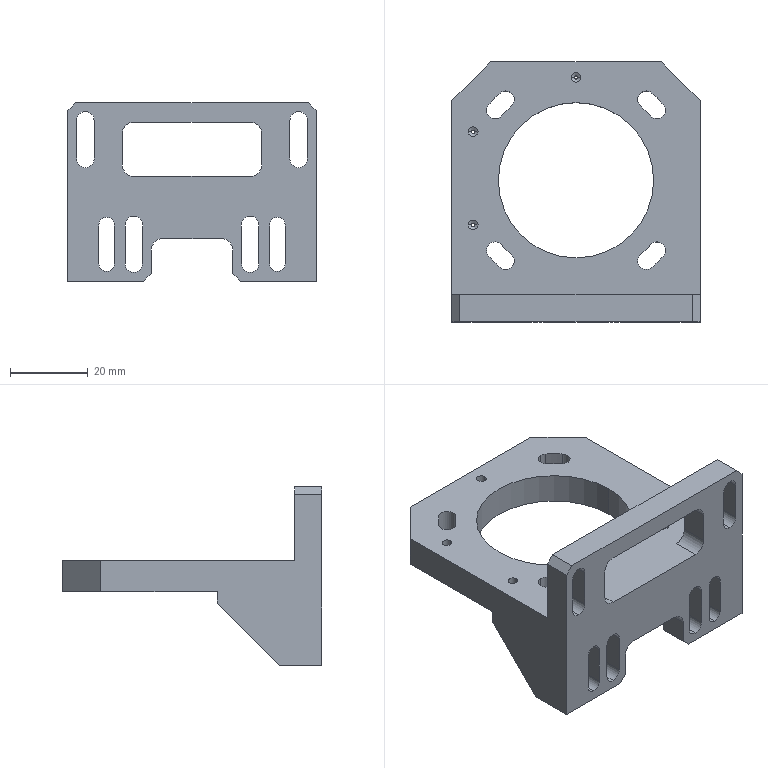NC program | NX | posted with a generic post | part box 64 x 67 x 46 mm
Lines 1 to 517 of 30645:
N10 G17 G21 G94 G90
(FLOOR_WALL_COPY , TOOL : D63)
N12 T02 M6
N14 G54
N16 G17 G0 G90 X-70. Y31.997 B0. C0. S2000 M3
N18 G43 Z30. H2
N20 Z6.9
N22 G94 G1 Z3.9 F1250.
N24 X-65.
N26 X65.
N28 Y12.599
N30 X-65.
N32 Y-6.8
N34 X65.
N36 X70.
N38 Z6.9
N40 G0 Z30.
N42 X-70. Y31.997
N44 Z6.8
N46 G1 Z3.8
N48 X-65.
N50 X65.
N52 Y12.599
N54 X-65.
N56 Y-6.8
N58 X65.
N60 X70.
N62 Z6.8
N64 G0 Z30.
N66 X-70. Y31.997
N68 Z6.7
N70 G1 Z3.7
N72 X-65.
N74 X65.
N76 Y12.599
N78 X-65.
N80 Y-6.8
N82 X65.
N84 X70.
N86 Z6.7
N88 G0 Z30.
N90 X-70. Y31.997
N92 Z6.6
N94 G1 Z3.6
N96 X-65.
N98 X65.
N100 Y12.599
N102 X-65.
N104 Y-6.8
N106 X65.
N108 X70.
N110 Z6.6
N112 G0 Z30.
N114 X-70. Y31.997
N116 Z6.5
N118 G1 Z3.5
N120 X-65.
N122 X65.
N124 Y12.599
N126 X-65.
N128 Y-6.8
N130 X65.
N132 X70.
N134 Z6.5
N136 G0 Z30.
N138 X-70. Y31.997
N140 Z6.4
N142 G1 Z3.4
N144 X-65.
N146 X65.
N148 Y12.599
N150 X-65.
N152 Y-6.8
N154 X65.
N156 X70.
N158 Z6.4
N160 G0 Z30.
N162 X-70. Y31.997
N164 Z6.3
N166 G1 Z3.3
N168 X-65.
N170 X65.
N172 Y12.599
N174 X-65.
N176 Y-6.8
N178 X65.
N180 X70.
N182 Z6.3
N184 G0 Z30.
N186 X-70. Y31.997
N188 Z6.2
N190 G1 Z3.2
N192 X-65.
N194 X65.
N196 Y12.599
N198 X-65.
N200 Y-6.8
N202 X65.
N204 X70.
N206 Z6.2
N208 G0 Z30.
N210 X-70. Y31.997
N212 Z6.1
N214 G1 Z3.1
N216 X-65.
N218 X65.
N220 Y12.599
N222 X-65.
N224 Y-6.8
N226 X65.
N228 X70.
N230 Z6.1
N232 G0 Z30.
N234 X-70. Y31.997
N236 Z6.
N238 G1 Z3.
N240 X-65.
N242 X65.
N244 Y12.599
N246 X-65.
N248 Y-6.8
N250 X65.
N252 X70.
N254 Z6.
N256 G0 Z30.
N258 X-70. Y31.997
N260 Z5.9
N262 G1 Z2.9
N264 X-65.
N266 X65.
N268 Y12.599
N270 X-65.
N272 Y-6.8
N274 X65.
N276 X70.
N278 Z5.9
N280 G0 Z30.
N282 X-70. Y31.997
N284 Z5.8
N286 G1 Z2.8
N288 X-65.
N290 X65.
N292 Y12.599
N294 X-65.
N296 Y-6.8
N298 X65.
N300 X70.
N302 Z5.8
N304 G0 Z30.
N306 X-70. Y31.997
N308 Z5.7
N310 G1 Z2.7
N312 X-65.
N314 X65.
N316 Y12.599
N318 X-65.
N320 Y-6.8
N322 X65.
N324 X70.
N326 Z5.7
N328 G0 Z30.
N330 X-70. Y31.997
N332 Z5.6
N334 G1 Z2.6
N336 X-65.
N338 X65.
N340 Y12.599
N342 X-65.
N344 Y-6.8
N346 X65.
N348 X70.
N350 Z5.6
N352 G0 Z30.
N354 X-70. Y31.997
N356 Z5.5
N358 G1 Z2.5
N360 X-65.
N362 X65.
N364 Y12.599
N366 X-65.
N368 Y-6.8
N370 X65.
N372 X70.
N374 Z5.5
N376 G0 Z30.
N378 X-70. Y31.997
N380 Z5.4
N382 G1 Z2.4
N384 X-65.
N386 X65.
N388 Y12.599
N390 X-65.
N392 Y-6.8
N394 X65.
N396 X70.
N398 Z5.4
N400 G0 Z30.
N402 X-70. Y31.997
N404 Z5.3
N406 G1 Z2.3
N408 X-65.
N410 X65.
N412 Y12.599
N414 X-65.
N416 Y-6.8
N418 X65.
N420 X70.
N422 Z5.3
N424 G0 Z30.
N426 X-70. Y31.997
N428 Z5.2
N430 G1 Z2.2
N432 X-65.
N434 X65.
N436 Y12.599
N438 X-65.
N440 Y-6.8
N442 X65.
N444 X70.
N446 Z5.2
N448 G0 Z30.
N450 X-70. Y31.997
N452 Z5.1
N454 G1 Z2.1
N456 X-65.
N458 X65.
N460 Y12.599
N462 X-65.
N464 Y-6.8
N466 X65.
N468 X70.
N470 Z5.1
N472 G0 Z30.
N474 X-70. Y31.997
N476 Z5.
N478 G1 Z2.
N480 X-65.
N482 X65.
N484 Y12.599
N486 X-65.
N488 Y-6.8
N490 X65.
N492 X70.
N494 Z5.
N496 G0 Z30.
N498 X-70. Y31.997
N500 Z4.9
N502 G1 Z1.9
N504 X-65.
N506 X65.
N508 Y12.599
N510 X-65.
N512 Y-6.8
N514 X65.
N516 X70.
N518 Z4.9
N520 G0 Z30.
N522 X-70. Y31.997
N524 Z4.8
N526 G1 Z1.8
N528 X-65.
N530 X65.
N532 Y12.599
N534 X-65.
N536 Y-6.8
N538 X65.
N540 X70.
N542 Z4.8
N544 G0 Z30.
N546 X-70. Y31.997
N548 Z4.7
N550 G1 Z1.7
N552 X-65.
N554 X65.
N556 Y12.599
N558 X-65.
N560 Y-6.8
N562 X65.
N564 X70.
N566 Z4.7
N568 G0 Z30.
N570 X-70. Y31.997
N572 Z4.6
N574 G1 Z1.6
N576 X-65.
N578 X65.
N580 Y12.599
N582 X-65.
N584 Y-6.8
N586 X65.
N588 X70.
N590 Z4.6
N592 G0 Z30.
N594 X-70. Y31.997
N596 Z4.5
N598 G1 Z1.5
N600 X-65.
N602 X65.
N604 Y12.599
N606 X-65.
N608 Y-6.8
N610 X65.
N612 X70.
N614 Z4.5
N616 G0 Z30.
N618 X-70. Y31.997
N620 Z4.4
N622 G1 Z1.4
N624 X-65.
N626 X65.
N628 Y12.599
N630 X-65.
N632 Y-6.8
N634 X65.
N636 X70.
N638 Z4.4
N640 G0 Z30.
N642 X-70. Y31.997
N644 Z4.3
N646 G1 Z1.3
N648 X-65.
N650 X65.
N652 Y12.599
N654 X-65.
N656 Y-6.8
N658 X65.
N660 X70.
N662 Z4.3
N664 G0 Z30.
N666 X-70. Y31.997
N668 Z4.2
N670 G1 Z1.2
N672 X-65.
N674 X65.
N676 Y12.599
N678 X-65.
N680 Y-6.8
N682 X65.
N684 X70.
N686 Z4.2
N688 G0 Z30.
N690 X-70. Y31.997
N692 Z4.1
N694 G1 Z1.1
N696 X-65.
N698 X65.
N700 Y12.599
N702 X-65.
N704 Y-6.8
N706 X65.
N708 X70.
N710 Z4.1
N712 G0 Z30.
N714 X-70. Y31.997
N716 Z4.
N718 G1 Z1.
N720 X-65.
N722 X65.
N724 Y12.599
N726 X-65.
N728 Y-6.8
N730 X65.
N732 X70.
N734 Z4.
N736 G0 Z30.
N738 X-70. Y31.997
N740 Z3.9
N742 G1 Z0.9
N744 X-65.
N746 X65.
N748 Y12.599
N750 X-65.
N752 Y-6.8
N754 X65.
N756 X70.
N758 Z3.9
N760 G0 Z30.
N762 X-70. Y31.997
N764 Z3.8
N766 G1 Z0.8
N768 X-65.
N770 X65.
N772 Y12.599
N774 X-65.
N776 Y-6.8
N778 X65.
N780 X70.
N782 Z3.8
N784 G0 Z30.
N786 X-70. Y31.997
N788 Z3.7
N790 G1 Z0.7
N792 X-65.
N794 X65.
N796 Y12.599
N798 X-65.
N800 Y-6.8
N802 X65.
N804 X70.
N806 Z3.7
N808 G0 Z30.
N810 X-70. Y31.997
N812 Z3.6
N814 G1 Z0.6
N816 X-65.
N818 X65.
N820 Y12.599
N822 X-65.
N824 Y-6.8
N826 X65.
N828 X70.
N830 Z3.6
N832 G0 Z30.
N834 X-70. Y31.997
N836 Z3.5
N838 G1 Z0.5
N840 X-65.
N842 X65.
N844 Y12.599
N846 X-65.
N848 Y-6.8
N850 X65.
N852 X70.
N854 Z3.5
N856 G0 Z30.
N858 X-70. Y31.997
N860 Z3.4
N862 G1 Z0.4
N864 X-65.
N866 X65.
N868 Y12.599
N870 X-65.
N872 Y-6.8
N874 X65.
N876 X70.
N878 Z3.4
N880 G0 Z30.
N882 X-70. Y31.997
N884 Z3.3
N886 G1 Z0.3
N888 X-65.
N890 X65.
N892 Y12.599
N894 X-65.
N896 Y-6.8
N898 X65.
N900 X70.
N902 Z3.3
N904 G0 Z30.
N906 X-70. Y31.997
N908 Z3.2
N910 G1 Z0.2
N912 X-65.
N914 X65.
N916 Y12.599
N918 X-65.
N920 Y-6.8
N922 X65.
N924 X70.
N926 Z3.2
N928 G0 Z30.
N930 X-70. Y31.997
N932 Z3.1
N934 G1 Z0.1
N936 X-65.
N938 X65.
N940 Y12.599
N942 X-65.
N944 Y-6.8
N946 X65.
N948 X70.
N950 Z3.1
N952 G0 Z30.
N954 M5
(FLOOR_WALL_COPY_COPY , TOOL : D10JING)
N956 T11 M6
N958 G54
N960 G17 G0 G90 X-43.5 Y31.997 B0. C0. S5000 M3
N962 G43 Z30. H11
N964 Z3.
N966 G94 G1 Z0. F1250.
N968 X-38.5
N970 X38.5
N972 Y26.997
N974 X-38.5
N976 Y21.997
N978 X38.5
N980 Y16.998
N982 X-38.5
N984 Y11.998
N986 X38.5
N988 Y6.998
N990 X-38.5
N992 Y1.999
N994 X38.5
N996 Y-3.001
N998 X-38.5
N1000 Y-8.001
N1002 X38.5
N1004 Y-13.001
N1006 X-38.5
N1008 Y-18.
N1010 X38.5
N1012 Y-23.
N1014 X-38.5
N1016 Y-28.
N1018 X38.5
N1020 X43.5
N1022 Z3.
N1024 G0 Z30.
N1026 M5